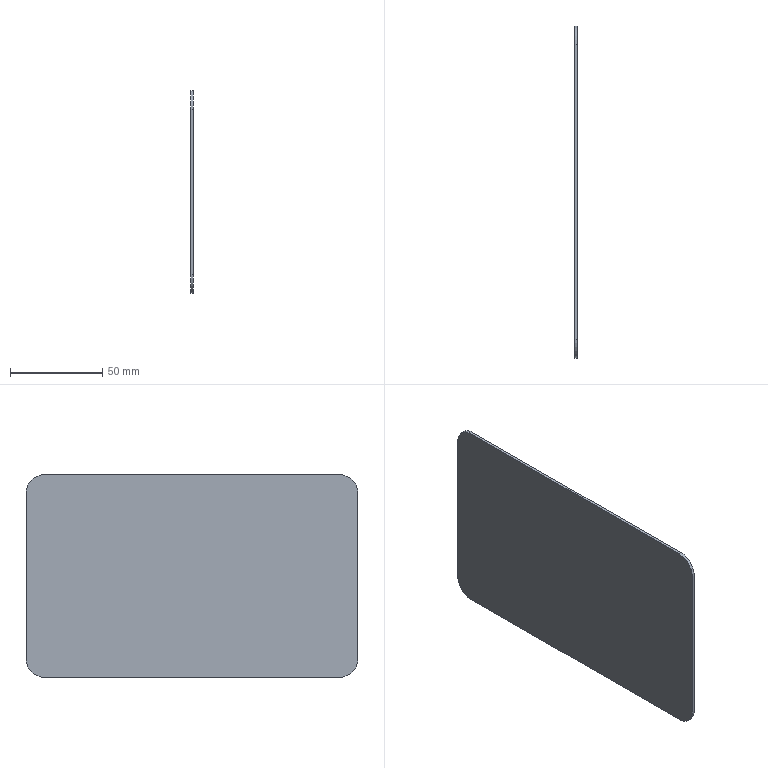Part | STEP file | RJWD-DY-B1_X2_5FEB5E7267DC680_1 | 1 solid | 10 faces | box 1.5 x 180 x 110 mm | volume 29571 mm3 | plane 6 | cylinder 4 | commonest cylinder face diameters 20 x4
STEP:
#1=CARTESIAN_POINT('',(0.,0.,0.));
#2=DIRECTION('',(0.,0.,1.));
#3=DIRECTION('',(1.,0.,0.));
#4=AXIS2_PLACEMENT_3D('',#1,#2,#3);
#5=CARTESIAN_POINT('',(768.8,3170.8,1288.594));
#6=VERTEX_POINT('',#5);
#7=CARTESIAN_POINT('',(768.8,3170.8,1378.594));
#8=VERTEX_POINT('',#7);
#9=CARTESIAN_POINT('',(768.8,3170.8,1288.594));
#10=DIRECTION('',(0.,0.,1.));
#11=VECTOR('',#10,1.);
#12=LINE('',#9,#11);
#13=CARTESIAN_POINT('',(770.3,3170.8,1378.594));
#14=DIRECTION('',(0.,1.,0.));
#15=DIRECTION('',(0.,0.,1.));
#16=AXIS2_PLACEMENT_3D('',#13,#14,#15);
#17=PLANE('',#16);
#18=CARTESIAN_POINT('',(-90.,-1.5));
#19=DIRECTION('',(1.,0.));
#20=VECTOR('',#19,1.);
#21=LINE('',#18,#20);
#22=(GEOMETRIC_REPRESENTATION_CONTEXT(2)PARAMETRIC_REPRESENTATION_CONTEXT()REPRESENTATION_CONTEXT('',''));
#23=DEFINITIONAL_REPRESENTATION('',(#21),#22);
#24=PCURVE('',#17,#23);
#25=CARTESIAN_POINT('',(768.8,3180.8,1288.594));
#26=DIRECTION('',(1.,0.,0.));
#27=DIRECTION('',(0.,0.,-1.));
#28=AXIS2_PLACEMENT_3D('',#25,#26,#27);
#29=PLANE('',#28);
#30=CARTESIAN_POINT('',(0.,-10.));
#31=DIRECTION('',(-1.,0.));
#32=VECTOR('',#31,1.);
#33=LINE('',#30,#32);
#34=(GEOMETRIC_REPRESENTATION_CONTEXT(2)PARAMETRIC_REPRESENTATION_CONTEXT()REPRESENTATION_CONTEXT('',''));
#35=DEFINITIONAL_REPRESENTATION('',(#33),#34);
#36=PCURVE('',#29,#35);
#37=SURFACE_CURVE('',#12,(#24,#36),.PCURVE_S1.);
#38=EDGE_CURVE('',#6,#8,#37,.T.);
#39=ORIENTED_EDGE('',*,*,#38,.T.);
#40=CARTESIAN_POINT('',(770.3,3170.8,1378.594));
#41=VERTEX_POINT('',#40);
#42=CARTESIAN_POINT('',(768.8,3170.8,1378.594));
#43=DIRECTION('',(1.,0.,0.));
#44=VECTOR('',#43,1.);
#45=LINE('',#42,#44);
#46=CARTESIAN_POINT('',(0.,-1.5));
#47=DIRECTION('',(0.,1.));
#48=VECTOR('',#47,1.);
#49=LINE('',#46,#48);
#50=(GEOMETRIC_REPRESENTATION_CONTEXT(2)PARAMETRIC_REPRESENTATION_CONTEXT()REPRESENTATION_CONTEXT('',''));
#51=DEFINITIONAL_REPRESENTATION('',(#49),#50);
#52=PCURVE('',#17,#51);
#53=CARTESIAN_POINT('',(770.3,3180.8,1378.594));
#54=DIRECTION('',(-1.,0.,0.));
#55=DIRECTION('',(0.,0.,1.));
#56=AXIS2_PLACEMENT_3D('',#53,#54,#55);
#57=CYLINDRICAL_SURFACE('',#56,10.);
#58=CARTESIAN_POINT('',(4.712,1.5));
#59=DIRECTION('',(0.,-1.));
#60=VECTOR('',#59,1.);
#61=LINE('',#58,#60);
#62=(GEOMETRIC_REPRESENTATION_CONTEXT(2)PARAMETRIC_REPRESENTATION_CONTEXT()REPRESENTATION_CONTEXT('',''));
#63=DEFINITIONAL_REPRESENTATION('',(#61),#62);
#64=PCURVE('',#57,#63);
#65=SURFACE_CURVE('',#45,(#52,#64),.PCURVE_S1.);
#66=EDGE_CURVE('',#8,#41,#65,.T.);
#67=ORIENTED_EDGE('',*,*,#66,.T.);
#68=CARTESIAN_POINT('',(770.3,3170.8,1288.594));
#69=VERTEX_POINT('',#68);
#70=CARTESIAN_POINT('',(770.3,3170.8,1288.594));
#71=DIRECTION('',(0.,0.,1.));
#72=VECTOR('',#71,1.);
#73=LINE('',#70,#72);
#74=CARTESIAN_POINT('',(-90.,0.));
#75=DIRECTION('',(1.,0.));
#76=VECTOR('',#75,1.);
#77=LINE('',#74,#76);
#78=(GEOMETRIC_REPRESENTATION_CONTEXT(2)PARAMETRIC_REPRESENTATION_CONTEXT()REPRESENTATION_CONTEXT('',''));
#79=DEFINITIONAL_REPRESENTATION('',(#77),#78);
#80=PCURVE('',#17,#79);
#81=CARTESIAN_POINT('',(770.3,3180.8,1288.594));
#82=DIRECTION('',(1.,0.,0.));
#83=DIRECTION('',(0.,0.,-1.));
#84=AXIS2_PLACEMENT_3D('',#81,#82,#83);
#85=PLANE('',#84);
#86=CARTESIAN_POINT('',(0.,-10.));
#87=DIRECTION('',(-1.,0.));
#88=VECTOR('',#87,1.);
#89=LINE('',#86,#88);
#90=(GEOMETRIC_REPRESENTATION_CONTEXT(2)PARAMETRIC_REPRESENTATION_CONTEXT()REPRESENTATION_CONTEXT('',''));
#91=DEFINITIONAL_REPRESENTATION('',(#89),#90);
#92=PCURVE('',#85,#91);
#93=SURFACE_CURVE('',#73,(#80,#92),.PCURVE_S1.);
#94=EDGE_CURVE('',#69,#41,#93,.T.);
#95=ORIENTED_EDGE('',*,*,#94,.F.);
#96=CARTESIAN_POINT('',(770.3,3170.8,1288.594));
#97=DIRECTION('',(-1.,0.,0.));
#98=VECTOR('',#97,1.);
#99=LINE('',#96,#98);
#100=CARTESIAN_POINT('',(-90.,0.));
#101=DIRECTION('',(0.,-1.));
#102=VECTOR('',#101,1.);
#103=LINE('',#100,#102);
#104=(GEOMETRIC_REPRESENTATION_CONTEXT(2)PARAMETRIC_REPRESENTATION_CONTEXT()REPRESENTATION_CONTEXT('',''));
#105=DEFINITIONAL_REPRESENTATION('',(#103),#104);
#106=PCURVE('',#17,#105);
#107=CARTESIAN_POINT('',(770.3,3180.8,1288.594));
#108=DIRECTION('',(-1.,0.,0.));
#109=DIRECTION('',(0.,0.,1.));
#110=AXIS2_PLACEMENT_3D('',#107,#108,#109);
#111=CYLINDRICAL_SURFACE('',#110,10.);
#112=CARTESIAN_POINT('',(4.712,0.));
#113=DIRECTION('',(0.,1.));
#114=VECTOR('',#113,1.);
#115=LINE('',#112,#114);
#116=(GEOMETRIC_REPRESENTATION_CONTEXT(2)PARAMETRIC_REPRESENTATION_CONTEXT()REPRESENTATION_CONTEXT('',''));
#117=DEFINITIONAL_REPRESENTATION('',(#115),#116);
#118=PCURVE('',#111,#117);
#119=SURFACE_CURVE('',#99,(#106,#118),.PCURVE_S1.);
#120=EDGE_CURVE('',#69,#6,#119,.T.);
#121=ORIENTED_EDGE('',*,*,#120,.T.);
#122=EDGE_LOOP('',(#39,#67,#95,#121));
#123=FACE_BOUND('',#122,.F.);
#124=ADVANCED_FACE('',(#123),#17,.F.);
#125=ORIENTED_EDGE('',*,*,#38,.F.);
#126=CARTESIAN_POINT('',(768.8,3180.8,1278.594));
#127=VERTEX_POINT('',#126);
#128=CARTESIAN_POINT('',(768.8,3180.8,1288.594));
#129=DIRECTION('',(-1.,0.,0.));
#130=DIRECTION('',(0.,0.,-1.));
#131=AXIS2_PLACEMENT_3D('',#128,#129,#130);
#132=CIRCLE('',#131,10.);
#133=CARTESIAN_POINT('',(10.,0.));
#134=CARTESIAN_POINT('',(10.,-17.321));
#135=CARTESIAN_POINT('',(-5.,-8.66));
#136=CARTESIAN_POINT('',(-20.,0.));
#137=CARTESIAN_POINT('',(-5.,8.66));
#138=CARTESIAN_POINT('',(10.,17.321));
#139=CARTESIAN_POINT('',(10.,0.));
#140=(BOUNDED_CURVE()B_SPLINE_CURVE(2,(#133,#134,#135,#136,#137,#138,#139),.UNSPECIFIED.,.T.,.F.)B_SPLINE_CURVE_WITH_KNOTS((1,2,2,2,2,1),(-2.094,0.,2.094,4.189,6.283,8.378),.UNSPECIFIED.)CURVE()GEOMETRIC_REPRESENTATION_ITEM()RATIONAL_B_SPLINE_CURVE((1.,0.5,1.,0.5,1.,0.5,1.))REPRESENTATION_ITEM(''));
#141=(GEOMETRIC_REPRESENTATION_CONTEXT(2)PARAMETRIC_REPRESENTATION_CONTEXT()REPRESENTATION_CONTEXT('',''));
#142=DEFINITIONAL_REPRESENTATION('',(#140),#141);
#143=PCURVE('',#29,#142);
#144=CARTESIAN_POINT('',(3.142,1.5));
#145=DIRECTION('',(1.,0.));
#146=VECTOR('',#145,1.);
#147=LINE('',#144,#146);
#148=(GEOMETRIC_REPRESENTATION_CONTEXT(2)PARAMETRIC_REPRESENTATION_CONTEXT()REPRESENTATION_CONTEXT('',''));
#149=DEFINITIONAL_REPRESENTATION('',(#147),#148);
#150=PCURVE('',#111,#149);
#151=SURFACE_CURVE('',#132,(#143,#150),.PCURVE_S1.);
#152=EDGE_CURVE('',#127,#6,#151,.T.);
#153=ORIENTED_EDGE('',*,*,#152,.F.);
#154=CARTESIAN_POINT('',(768.8,3340.8,1278.594));
#155=VERTEX_POINT('',#154);
#156=CARTESIAN_POINT('',(768.8,3340.8,1278.594));
#157=DIRECTION('',(0.,-1.,0.));
#158=VECTOR('',#157,1.);
#159=LINE('',#156,#158);
#160=CARTESIAN_POINT('',(10.,160.));
#161=DIRECTION('',(0.,-1.));
#162=VECTOR('',#161,1.);
#163=LINE('',#160,#162);
#164=(GEOMETRIC_REPRESENTATION_CONTEXT(2)PARAMETRIC_REPRESENTATION_CONTEXT()REPRESENTATION_CONTEXT('',''));
#165=DEFINITIONAL_REPRESENTATION('',(#163),#164);
#166=PCURVE('',#29,#165);
#167=CARTESIAN_POINT('',(770.3,3180.8,1278.594));
#168=DIRECTION('',(0.,0.,1.));
#169=DIRECTION('',(1.,0.,0.));
#170=AXIS2_PLACEMENT_3D('',#167,#168,#169);
#171=PLANE('',#170);
#172=CARTESIAN_POINT('',(-1.5,160.));
#173=DIRECTION('',(0.,-1.));
#174=VECTOR('',#173,1.);
#175=LINE('',#172,#174);
#176=(GEOMETRIC_REPRESENTATION_CONTEXT(2)PARAMETRIC_REPRESENTATION_CONTEXT()REPRESENTATION_CONTEXT('',''));
#177=DEFINITIONAL_REPRESENTATION('',(#175),#176);
#178=PCURVE('',#171,#177);
#179=SURFACE_CURVE('',#159,(#166,#178),.PCURVE_S1.);
#180=EDGE_CURVE('',#155,#127,#179,.T.);
#181=ORIENTED_EDGE('',*,*,#180,.F.);
#182=CARTESIAN_POINT('',(768.8,3350.8,1288.594));
#183=VERTEX_POINT('',#182);
#184=CARTESIAN_POINT('',(768.8,3340.8,1288.594));
#185=DIRECTION('',(-1.,0.,0.));
#186=DIRECTION('',(0.,1.,0.));
#187=AXIS2_PLACEMENT_3D('',#184,#185,#186);
#188=CIRCLE('',#187,10.);
#189=CARTESIAN_POINT('',(0.,170.));
#190=CARTESIAN_POINT('',(17.321,170.));
#191=CARTESIAN_POINT('',(8.66,155.));
#192=CARTESIAN_POINT('',(0.,140.));
#193=CARTESIAN_POINT('',(-8.66,155.));
#194=CARTESIAN_POINT('',(-17.321,170.));
#195=CARTESIAN_POINT('',(0.,170.));
#196=(BOUNDED_CURVE()B_SPLINE_CURVE(2,(#189,#190,#191,#192,#193,#194,#195),.UNSPECIFIED.,.T.,.F.)B_SPLINE_CURVE_WITH_KNOTS((1,2,2,2,2,1),(-2.094,0.,2.094,4.189,6.283,8.378),.UNSPECIFIED.)CURVE()GEOMETRIC_REPRESENTATION_ITEM()RATIONAL_B_SPLINE_CURVE((1.,0.5,1.,0.5,1.,0.5,1.))REPRESENTATION_ITEM(''));
#197=(GEOMETRIC_REPRESENTATION_CONTEXT(2)PARAMETRIC_REPRESENTATION_CONTEXT()REPRESENTATION_CONTEXT('',''));
#198=DEFINITIONAL_REPRESENTATION('',(#196),#197);
#199=PCURVE('',#29,#198);
#200=CARTESIAN_POINT('',(770.3,3340.8,1288.594));
#201=DIRECTION('',(-1.,0.,0.));
#202=DIRECTION('',(0.,0.,1.));
#203=AXIS2_PLACEMENT_3D('',#200,#201,#202);
#204=CYLINDRICAL_SURFACE('',#203,10.);
#205=CARTESIAN_POINT('',(1.571,1.5));
#206=DIRECTION('',(1.,0.));
#207=VECTOR('',#206,1.);
#208=LINE('',#205,#207);
#209=(GEOMETRIC_REPRESENTATION_CONTEXT(2)PARAMETRIC_REPRESENTATION_CONTEXT()REPRESENTATION_CONTEXT('',''));
#210=DEFINITIONAL_REPRESENTATION('',(#208),#209);
#211=PCURVE('',#204,#210);
#212=SURFACE_CURVE('',#188,(#199,#211),.PCURVE_S1.);
#213=EDGE_CURVE('',#183,#155,#212,.T.);
#214=ORIENTED_EDGE('',*,*,#213,.F.);
#215=CARTESIAN_POINT('',(768.8,3350.8,1378.594));
#216=VERTEX_POINT('',#215);
#217=CARTESIAN_POINT('',(768.8,3350.8,1378.594));
#218=DIRECTION('',(0.,0.,-1.));
#219=VECTOR('',#218,1.);
#220=LINE('',#217,#219);
#221=CARTESIAN_POINT('',(-90.,170.));
#222=DIRECTION('',(1.,0.));
#223=VECTOR('',#222,1.);
#224=LINE('',#221,#223);
#225=(GEOMETRIC_REPRESENTATION_CONTEXT(2)PARAMETRIC_REPRESENTATION_CONTEXT()REPRESENTATION_CONTEXT('',''));
#226=DEFINITIONAL_REPRESENTATION('',(#224),#225);
#227=PCURVE('',#29,#226);
#228=CARTESIAN_POINT('',(770.3,3350.8,1288.594));
#229=DIRECTION('',(0.,-1.,0.));
#230=DIRECTION('',(0.,0.,-1.));
#231=AXIS2_PLACEMENT_3D('',#228,#229,#230);
#232=PLANE('',#231);
#233=CARTESIAN_POINT('',(-90.,-1.5));
#234=DIRECTION('',(1.,0.));
#235=VECTOR('',#234,1.);
#236=LINE('',#233,#235);
#237=(GEOMETRIC_REPRESENTATION_CONTEXT(2)PARAMETRIC_REPRESENTATION_CONTEXT()REPRESENTATION_CONTEXT('',''));
#238=DEFINITIONAL_REPRESENTATION('',(#236),#237);
#239=PCURVE('',#232,#238);
#240=SURFACE_CURVE('',#220,(#227,#239),.PCURVE_S1.);
#241=EDGE_CURVE('',#216,#183,#240,.T.);
#242=ORIENTED_EDGE('',*,*,#241,.F.);
#243=CARTESIAN_POINT('',(768.8,3340.8,1388.594));
#244=VERTEX_POINT('',#243);
#245=CARTESIAN_POINT('',(768.8,3340.8,1378.594));
#246=DIRECTION('',(-1.,0.,0.));
#247=DIRECTION('',(0.,0.,1.));
#248=AXIS2_PLACEMENT_3D('',#245,#246,#247);
#249=CIRCLE('',#248,10.);
#250=CARTESIAN_POINT('',(-100.,160.));
#251=CARTESIAN_POINT('',(-100.,177.321));
#252=CARTESIAN_POINT('',(-85.,168.66));
#253=CARTESIAN_POINT('',(-70.,160.));
#254=CARTESIAN_POINT('',(-85.,151.34));
#255=CARTESIAN_POINT('',(-100.,142.679));
#256=CARTESIAN_POINT('',(-100.,160.));
#257=(BOUNDED_CURVE()B_SPLINE_CURVE(2,(#250,#251,#252,#253,#254,#255,#256),.UNSPECIFIED.,.T.,.F.)B_SPLINE_CURVE_WITH_KNOTS((1,2,2,2,2,1),(-2.094,0.,2.094,4.189,6.283,8.378),.UNSPECIFIED.)CURVE()GEOMETRIC_REPRESENTATION_ITEM()RATIONAL_B_SPLINE_CURVE((1.,0.5,1.,0.5,1.,0.5,1.))REPRESENTATION_ITEM(''));
#258=(GEOMETRIC_REPRESENTATION_CONTEXT(2)PARAMETRIC_REPRESENTATION_CONTEXT()REPRESENTATION_CONTEXT('',''));
#259=DEFINITIONAL_REPRESENTATION('',(#257),#258);
#260=PCURVE('',#29,#259);
#261=CARTESIAN_POINT('',(770.3,3340.8,1378.594));
#262=DIRECTION('',(-1.,0.,0.));
#263=DIRECTION('',(0.,0.,1.));
#264=AXIS2_PLACEMENT_3D('',#261,#262,#263);
#265=CYLINDRICAL_SURFACE('',#264,10.);
#266=CARTESIAN_POINT('',(0.,1.5));
#267=DIRECTION('',(1.,0.));
#268=VECTOR('',#267,1.);
#269=LINE('',#266,#268);
#270=(GEOMETRIC_REPRESENTATION_CONTEXT(2)PARAMETRIC_REPRESENTATION_CONTEXT()REPRESENTATION_CONTEXT('',''));
#271=DEFINITIONAL_REPRESENTATION('',(#269),#270);
#272=PCURVE('',#265,#271);
#273=SURFACE_CURVE('',#249,(#260,#272),.PCURVE_S1.);
#274=EDGE_CURVE('',#244,#216,#273,.T.);
#275=ORIENTED_EDGE('',*,*,#274,.F.);
#276=CARTESIAN_POINT('',(768.8,3180.8,1388.594));
#277=VERTEX_POINT('',#276);
#278=CARTESIAN_POINT('',(768.8,3180.8,1388.594));
#279=DIRECTION('',(0.,1.,0.));
#280=VECTOR('',#279,1.);
#281=LINE('',#278,#280);
#282=CARTESIAN_POINT('',(-100.,0.));
#283=DIRECTION('',(0.,1.));
#284=VECTOR('',#283,1.);
#285=LINE('',#282,#284);
#286=(GEOMETRIC_REPRESENTATION_CONTEXT(2)PARAMETRIC_REPRESENTATION_CONTEXT()REPRESENTATION_CONTEXT('',''));
#287=DEFINITIONAL_REPRESENTATION('',(#285),#286);
#288=PCURVE('',#29,#287);
#289=CARTESIAN_POINT('',(770.3,3340.8,1388.594));
#290=DIRECTION('',(0.,0.,-1.));
#291=DIRECTION('',(-1.,0.,0.));
#292=AXIS2_PLACEMENT_3D('',#289,#290,#291);
#293=PLANE('',#292);
#294=CARTESIAN_POINT('',(1.5,-160.));
#295=DIRECTION('',(0.,1.));
#296=VECTOR('',#295,1.);
#297=LINE('',#294,#296);
#298=(GEOMETRIC_REPRESENTATION_CONTEXT(2)PARAMETRIC_REPRESENTATION_CONTEXT()REPRESENTATION_CONTEXT('',''));
#299=DEFINITIONAL_REPRESENTATION('',(#297),#298);
#300=PCURVE('',#293,#299);
#301=SURFACE_CURVE('',#281,(#288,#300),.PCURVE_S1.);
#302=EDGE_CURVE('',#277,#244,#301,.T.);
#303=ORIENTED_EDGE('',*,*,#302,.F.);
#304=CARTESIAN_POINT('',(768.8,3180.8,1378.594));
#305=DIRECTION('',(-1.,0.,0.));
#306=DIRECTION('',(0.,-1.,0.));
#307=AXIS2_PLACEMENT_3D('',#304,#305,#306);
#308=CIRCLE('',#307,10.);
#309=CARTESIAN_POINT('',(-90.,-10.));
#310=CARTESIAN_POINT('',(-107.321,-10.));
#311=CARTESIAN_POINT('',(-98.66,5.));
#312=CARTESIAN_POINT('',(-90.,20.));
#313=CARTESIAN_POINT('',(-81.34,5.));
#314=CARTESIAN_POINT('',(-72.679,-10.));
#315=CARTESIAN_POINT('',(-90.,-10.));
#316=(BOUNDED_CURVE()B_SPLINE_CURVE(2,(#309,#310,#311,#312,#313,#314,#315),.UNSPECIFIED.,.T.,.F.)B_SPLINE_CURVE_WITH_KNOTS((1,2,2,2,2,1),(-2.094,0.,2.094,4.189,6.283,8.378),.UNSPECIFIED.)CURVE()GEOMETRIC_REPRESENTATION_ITEM()RATIONAL_B_SPLINE_CURVE((1.,0.5,1.,0.5,1.,0.5,1.))REPRESENTATION_ITEM(''));
#317=(GEOMETRIC_REPRESENTATION_CONTEXT(2)PARAMETRIC_REPRESENTATION_CONTEXT()REPRESENTATION_CONTEXT('',''));
#318=DEFINITIONAL_REPRESENTATION('',(#316),#317);
#319=PCURVE('',#29,#318);
#320=CARTESIAN_POINT('',(4.712,1.5));
#321=DIRECTION('',(1.,0.));
#322=VECTOR('',#321,1.);
#323=LINE('',#320,#322);
#324=(GEOMETRIC_REPRESENTATION_CONTEXT(2)PARAMETRIC_REPRESENTATION_CONTEXT()REPRESENTATION_CONTEXT('',''));
#325=DEFINITIONAL_REPRESENTATION('',(#323),#324);
#326=PCURVE('',#57,#325);
#327=SURFACE_CURVE('',#308,(#319,#326),.PCURVE_S1.);
#328=EDGE_CURVE('',#8,#277,#327,.T.);
#329=ORIENTED_EDGE('',*,*,#328,.F.);
#330=EDGE_LOOP('',(#125,#153,#181,#214,#242,#275,#303,#329));
#331=FACE_BOUND('',#330,.F.);
#332=ADVANCED_FACE('',(#331),#29,.F.);
#333=CARTESIAN_POINT('',(770.3,3180.8,1278.594));
#334=VERTEX_POINT('',#333);
#335=CARTESIAN_POINT('',(768.8,3180.8,1278.594));
#336=DIRECTION('',(1.,0.,0.));
#337=VECTOR('',#336,1.);
#338=LINE('',#335,#337);
#339=CARTESIAN_POINT('',(3.142,1.5));
#340=DIRECTION('',(0.,-1.));
#341=VECTOR('',#340,1.);
#342=LINE('',#339,#341);
#343=(GEOMETRIC_REPRESENTATION_CONTEXT(2)PARAMETRIC_REPRESENTATION_CONTEXT()REPRESENTATION_CONTEXT('',''));
#344=DEFINITIONAL_REPRESENTATION('',(#342),#343);
#345=PCURVE('',#111,#344);
#346=CARTESIAN_POINT('',(-1.5,0.));
#347=DIRECTION('',(1.,0.));
#348=VECTOR('',#347,1.);
#349=LINE('',#346,#348);
#350=(GEOMETRIC_REPRESENTATION_CONTEXT(2)PARAMETRIC_REPRESENTATION_CONTEXT()REPRESENTATION_CONTEXT('',''));
#351=DEFINITIONAL_REPRESENTATION('',(#349),#350);
#352=PCURVE('',#171,#351);
#353=SURFACE_CURVE('',#338,(#345,#352),.PCURVE_S1.);
#354=EDGE_CURVE('',#127,#334,#353,.T.);
#355=ORIENTED_EDGE('',*,*,#354,.T.);
#356=CARTESIAN_POINT('',(770.3,3180.8,1288.594));
#357=DIRECTION('',(1.,0.,0.));
#358=DIRECTION('',(0.,-1.,0.));
#359=AXIS2_PLACEMENT_3D('',#356,#357,#358);
#360=CIRCLE('',#359,10.);
#361=CARTESIAN_POINT('',(4.712,0.));
#362=DIRECTION('',(-1.,0.));
#363=VECTOR('',#362,1.);
#364=LINE('',#361,#363);
#365=(GEOMETRIC_REPRESENTATION_CONTEXT(2)PARAMETRIC_REPRESENTATION_CONTEXT()REPRESENTATION_CONTEXT('',''));
#366=DEFINITIONAL_REPRESENTATION('',(#364),#365);
#367=PCURVE('',#111,#366);
#368=CARTESIAN_POINT('',(0.,0.));
#369=DIRECTION('',(0.,-1.));
#370=AXIS2_PLACEMENT_2D('',#368,#369);
#371=CIRCLE('',#370,10.);
#372=(GEOMETRIC_REPRESENTATION_CONTEXT(2)PARAMETRIC_REPRESENTATION_CONTEXT()REPRESENTATION_CONTEXT('',''));
#373=DEFINITIONAL_REPRESENTATION('',(#371),#372);
#374=PCURVE('',#85,#373);
#375=SURFACE_CURVE('',#360,(#367,#374),.PCURVE_S1.);
#376=EDGE_CURVE('',#69,#334,#375,.T.);
#377=ORIENTED_EDGE('',*,*,#376,.F.);
#378=ORIENTED_EDGE('',*,*,#120,.T.);
#379=ORIENTED_EDGE('',*,*,#152,.F.);
#380=EDGE_LOOP('',(#355,#377,#378,#379));
#381=FACE_BOUND('',#380,.T.);
#382=ADVANCED_FACE('',(#381),#111,.T.);
#383=ORIENTED_EDGE('',*,*,#94,.T.);
#384=CARTESIAN_POINT('',(770.3,3180.8,1388.594));
#385=VERTEX_POINT('',#384);
#386=CARTESIAN_POINT('',(770.3,3180.8,1378.594));
#387=DIRECTION('',(1.,0.,0.));
#388=DIRECTION('',(0.,0.,1.));
#389=AXIS2_PLACEMENT_3D('',#386,#387,#388);
#390=CIRCLE('',#389,10.);
#391=CARTESIAN_POINT('',(-90.,0.));
#392=DIRECTION('',(-1.,0.));
#393=AXIS2_PLACEMENT_2D('',#391,#392);
#394=CIRCLE('',#393,10.);
#395=(GEOMETRIC_REPRESENTATION_CONTEXT(2)PARAMETRIC_REPRESENTATION_CONTEXT()REPRESENTATION_CONTEXT('',''));
#396=DEFINITIONAL_REPRESENTATION('',(#394),#395);
#397=PCURVE('',#85,#396);
#398=CARTESIAN_POINT('',(6.283,0.));
#399=DIRECTION('',(-1.,0.));
#400=VECTOR('',#399,1.);
#401=LINE('',#398,#400);
#402=(GEOMETRIC_REPRESENTATION_CONTEXT(2)PARAMETRIC_REPRESENTATION_CONTEXT()REPRESENTATION_CONTEXT('',''));
#403=DEFINITIONAL_REPRESENTATION('',(#401),#402);
#404=PCURVE('',#57,#403);
#405=SURFACE_CURVE('',#390,(#397,#404),.PCURVE_S1.);
#406=EDGE_CURVE('',#385,#41,#405,.T.);
#407=ORIENTED_EDGE('',*,*,#406,.F.);
#408=CARTESIAN_POINT('',(770.3,3340.8,1388.594));
#409=VERTEX_POINT('',#408);
#410=CARTESIAN_POINT('',(770.3,3180.8,1388.594));
#411=DIRECTION('',(0.,1.,0.));
#412=VECTOR('',#411,1.);
#413=LINE('',#410,#412);
#414=CARTESIAN_POINT('',(-100.,0.));
#415=DIRECTION('',(0.,1.));
#416=VECTOR('',#415,1.);
#417=LINE('',#414,#416);
#418=(GEOMETRIC_REPRESENTATION_CONTEXT(2)PARAMETRIC_REPRESENTATION_CONTEXT()REPRESENTATION_CONTEXT('',''));
#419=DEFINITIONAL_REPRESENTATION('',(#417),#418);
#420=PCURVE('',#85,#419);
#421=CARTESIAN_POINT('',(0.,-160.));
#422=DIRECTION('',(0.,1.));
#423=VECTOR('',#422,1.);
#424=LINE('',#421,#423);
#425=(GEOMETRIC_REPRESENTATION_CONTEXT(2)PARAMETRIC_REPRESENTATION_CONTEXT()REPRESENTATION_CONTEXT('',''));
#426=DEFINITIONAL_REPRESENTATION('',(#424),#425);
#427=PCURVE('',#293,#426);
#428=SURFACE_CURVE('',#413,(#420,#427),.PCURVE_S1.);
#429=EDGE_CURVE('',#385,#409,#428,.T.);
#430=ORIENTED_EDGE('',*,*,#429,.T.);
#431=CARTESIAN_POINT('',(770.3,3350.8,1378.594));
#432=VERTEX_POINT('',#431);
#433=CARTESIAN_POINT('',(770.3,3340.8,1378.594));
#434=DIRECTION('',(1.,0.,0.));
#435=DIRECTION('',(0.,1.,0.));
#436=AXIS2_PLACEMENT_3D('',#433,#434,#435);
#437=CIRCLE('',#436,10.);
#438=CARTESIAN_POINT('',(-90.,160.));
#439=DIRECTION('',(0.,1.));
#440=AXIS2_PLACEMENT_2D('',#438,#439);
#441=CIRCLE('',#440,10.);
#442=(GEOMETRIC_REPRESENTATION_CONTEXT(2)PARAMETRIC_REPRESENTATION_CONTEXT()REPRESENTATION_CONTEXT('',''));
#443=DEFINITIONAL_REPRESENTATION('',(#441),#442);
#444=PCURVE('',#85,#443);
#445=CARTESIAN_POINT('',(1.571,0.));
#446=DIRECTION('',(-1.,0.));
#447=VECTOR('',#446,1.);
#448=LINE('',#445,#447);
#449=(GEOMETRIC_REPRESENTATION_CONTEXT(2)PARAMETRIC_REPRESENTATION_CONTEXT()REPRESENTATION_CONTEXT('',''));
#450=DEFINITIONAL_REPRESENTATION('',(#448),#449);
#451=PCURVE('',#265,#450);
#452=SURFACE_CURVE('',#437,(#444,#451),.PCURVE_S1.);
#453=EDGE_CURVE('',#432,#409,#452,.T.);
#454=ORIENTED_EDGE('',*,*,#453,.F.);
#455=CARTESIAN_POINT('',(770.3,3350.8,1288.594));
#456=VERTEX_POINT('',#455);
#457=CARTESIAN_POINT('',(770.3,3350.8,1378.594));
#458=DIRECTION('',(0.,0.,-1.));
#459=VECTOR('',#458,1.);
#460=LINE('',#457,#459);
#461=CARTESIAN_POINT('',(-90.,170.));
#462=DIRECTION('',(1.,0.));
#463=VECTOR('',#462,1.);
#464=LINE('',#461,#463);
#465=(GEOMETRIC_REPRESENTATION_CONTEXT(2)PARAMETRIC_REPRESENTATION_CONTEXT()REPRESENTATION_CONTEXT('',''));
#466=DEFINITIONAL_REPRESENTATION('',(#464),#465);
#467=PCURVE('',#85,#466);
#468=CARTESIAN_POINT('',(-90.,0.));
#469=DIRECTION('',(1.,0.));
#470=VECTOR('',#469,1.);
#471=LINE('',#468,#470);
#472=(GEOMETRIC_REPRESENTATION_CONTEXT(2)PARAMETRIC_REPRESENTATION_CONTEXT()REPRESENTATION_CONTEXT('',''));
#473=DEFINITIONAL_REPRESENTATION('',(#471),#472);
#474=PCURVE('',#232,#473);
#475=SURFACE_CURVE('',#460,(#467,#474),.PCURVE_S1.);
#476=EDGE_CURVE('',#432,#456,#475,.T.);
#477=ORIENTED_EDGE('',*,*,#476,.T.);
#478=CARTESIAN_POINT('',(770.3,3340.8,1278.594));
#479=VERTEX_POINT('',#478);
#480=CARTESIAN_POINT('',(770.3,3340.8,1288.594));
#481=DIRECTION('',(1.,0.,0.));
#482=DIRECTION('',(0.,0.,-1.));
#483=AXIS2_PLACEMENT_3D('',#480,#481,#482);
#484=CIRCLE('',#483,10.);
#485=CARTESIAN_POINT('',(0.,160.));
#486=DIRECTION('',(1.,0.));
#487=AXIS2_PLACEMENT_2D('',#485,#486);
#488=CIRCLE('',#487,10.);
#489=(GEOMETRIC_REPRESENTATION_CONTEXT(2)PARAMETRIC_REPRESENTATION_CONTEXT()REPRESENTATION_CONTEXT('',''));
#490=DEFINITIONAL_REPRESENTATION('',(#488),#489);
#491=PCURVE('',#85,#490);
#492=CARTESIAN_POINT('',(3.142,0.));
#493=DIRECTION('',(-1.,0.));
#494=VECTOR('',#493,1.);
#495=LINE('',#492,#494);
#496=(GEOMETRIC_REPRESENTATION_CONTEXT(2)PARAMETRIC_REPRESENTATION_CONTEXT()REPRESENTATION_CONTEXT('',''));
#497=DEFINITIONAL_REPRESENTATION('',(#495),#496);
#498=PCURVE('',#204,#497);
#499=SURFACE_CURVE('',#484,(#491,#498),.PCURVE_S1.);
#500=EDGE_CURVE('',#479,#456,#499,.T.);
#501=ORIENTED_EDGE('',*,*,#500,.F.);
#502=CARTESIAN_POINT('',(770.3,3340.8,1278.594));
#503=DIRECTION('',(0.,-1.,0.));
#504=VECTOR('',#503,1.);
#505=LINE('',#502,#504);
#506=CARTESIAN_POINT('',(10.,160.));
#507=DIRECTION('',(0.,-1.));
#508=VECTOR('',#507,1.);
#509=LINE('',#506,#508);
#510=(GEOMETRIC_REPRESENTATION_CONTEXT(2)PARAMETRIC_REPRESENTATION_CONTEXT()REPRESENTATION_CONTEXT('',''));
#511=DEFINITIONAL_REPRESENTATION('',(#509),#510);
#512=PCURVE('',#85,#511);
#513=CARTESIAN_POINT('',(0.,160.));
#514=DIRECTION('',(0.,-1.));
#515=VECTOR('',#514,1.);
#516=LINE('',#513,#515);
#517=(GEOMETRIC_REPRESENTATION_CONTEXT(2)PARAMETRIC_REPRESENTATION_CONTEXT()REPRESENTATION_CONTEXT('',''));
#518=DEFINITIONAL_REPRESENTATION('',(#516),#517);
#519=PCURVE('',#171,#518);
#520=SURFACE_CURVE('',#505,(#512,#519),.PCURVE_S1.);
#521=EDGE_CURVE('',#479,#334,#520,.T.);
#522=ORIENTED_EDGE('',*,*,#521,.T.);
#523=ORIENTED_EDGE('',*,*,#376,.F.);
#524=EDGE_LOOP('',(#383,#407,#430,#454,#477,#501,#522,#523));
#525=FACE_BOUND('',#524,.F.);
#526=ADVANCED_FACE('',(#525),#85,.T.);
#527=ORIENTED_EDGE('',*,*,#66,.T.);
#528=ORIENTED_EDGE('',*,*,#406,.F.);
#529=CARTESIAN_POINT('',(770.3,3180.8,1388.594));
#530=DIRECTION('',(-1.,0.,0.));
#531=VECTOR('',#530,1.);
#532=LINE('',#529,#531);
#533=CARTESIAN_POINT('',(6.283,0.));
#534=DIRECTION('',(0.,1.));
#535=VECTOR('',#534,1.);
#536=LINE('',#533,#535);
#537=(GEOMETRIC_REPRESENTATION_CONTEXT(2)PARAMETRIC_REPRESENTATION_CONTEXT()REPRESENTATION_CONTEXT('',''));
#538=DEFINITIONAL_REPRESENTATION('',(#536),#537);
#539=PCURVE('',#57,#538);
#540=CARTESIAN_POINT('',(0.,-160.));
#541=DIRECTION('',(1.,0.));
#542=VECTOR('',#541,1.);
#543=LINE('',#540,#542);
#544=(GEOMETRIC_REPRESENTATION_CONTEXT(2)PARAMETRIC_REPRESENTATION_CONTEXT()REPRESENTATION_CONTEXT('',''));
#545=DEFINITIONAL_REPRESENTATION('',(#543),#544);
#546=PCURVE('',#293,#545);
#547=SURFACE_CURVE('',#532,(#539,#546),.PCURVE_S1.);
#548=EDGE_CURVE('',#385,#277,#547,.T.);
#549=ORIENTED_EDGE('',*,*,#548,.T.);
#550=ORIENTED_EDGE('',*,*,#328,.F.);
#551=EDGE_LOOP('',(#527,#528,#549,#550));
#552=FACE_BOUND('',#551,.T.);
#553=ADVANCED_FACE('',(#552),#57,.T.);
#554=ORIENTED_EDGE('',*,*,#302,.T.);
#555=CARTESIAN_POINT('',(768.8,3340.8,1388.594));
#556=DIRECTION('',(1.,0.,0.));
#557=VECTOR('',#556,1.);
#558=LINE('',#555,#557);
#559=CARTESIAN_POINT('',(1.5,0.));
#560=DIRECTION('',(-1.,0.));
#561=VECTOR('',#560,1.);
#562=LINE('',#559,#561);
#563=(GEOMETRIC_REPRESENTATION_CONTEXT(2)PARAMETRIC_REPRESENTATION_CONTEXT()REPRESENTATION_CONTEXT('',''));
#564=DEFINITIONAL_REPRESENTATION('',(#562),#563);
#565=PCURVE('',#293,#564);
#566=CARTESIAN_POINT('',(0.,1.5));
#567=CARTESIAN_POINT('',(0.,1.477));
#568=CARTESIAN_POINT('',(0.,1.432));
#569=CARTESIAN_POINT('',(0.,1.364));
#570=CARTESIAN_POINT('',(0.,1.295));
#571=CARTESIAN_POINT('',(0.,1.227));
#572=CARTESIAN_POINT('',(0.,1.159));
#573=CARTESIAN_POINT('',(0.,1.091));
#574=CARTESIAN_POINT('',(0.,1.023));
#575=CARTESIAN_POINT('',(0.,0.9545));
#576=CARTESIAN_POINT('',(0.,0.8864));
#577=CARTESIAN_POINT('',(0.,0.8182));
#578=CARTESIAN_POINT('',(0.,0.75));
#579=CARTESIAN_POINT('',(0.,0.6818));
#580=CARTESIAN_POINT('',(0.,0.6136));
#581=CARTESIAN_POINT('',(0.,0.5455));
#582=CARTESIAN_POINT('',(0.,0.4773));
#583=CARTESIAN_POINT('',(0.,0.4091));
#584=CARTESIAN_POINT('',(0.,0.3409));
#585=CARTESIAN_POINT('',(0.,0.2727));
#586=CARTESIAN_POINT('',(0.,0.2045));
#587=CARTESIAN_POINT('',(0.,0.1364));
#588=CARTESIAN_POINT('',(0.,0.06818));
#589=CARTESIAN_POINT('',(0.,0.02273));
#590=CARTESIAN_POINT('',(0.,0.));
#591=B_SPLINE_CURVE_WITH_KNOTS('',3,(#566,#567,#568,#569,#570,#571,#572,#573,#574,#575,#576,#577,#578,#579,#580,#581,#582,#583,#584,#585,#586,#587,#588,#589,#590),.UNSPECIFIED.,.F.,.F.,(4,1,1,1,1,1,1,1,1,1,1,1,1,1,1,1,1,1,1,1,1,1,4),(0.,0.06818,0.1364,0.2045,0.2727,0.3409,0.4091,0.4773,0.5455,0.6136,0.6818,0.75,0.8182,0.8864,0.9545,1.023,1.091,1.159,1.227,1.295,1.364,1.432,1.5),.QUASI_UNIFORM_KNOTS.);
#592=(GEOMETRIC_REPRESENTATION_CONTEXT(2)PARAMETRIC_REPRESENTATION_CONTEXT()REPRESENTATION_CONTEXT('',''));
#593=DEFINITIONAL_REPRESENTATION('',(#591),#592);
#594=PCURVE('',#265,#593);
#595=SURFACE_CURVE('',#558,(#565,#594),.PCURVE_S1.);
#596=EDGE_CURVE('',#244,#409,#595,.T.);
#597=ORIENTED_EDGE('',*,*,#596,.T.);
#598=ORIENTED_EDGE('',*,*,#429,.F.);
#599=ORIENTED_EDGE('',*,*,#548,.T.);
#600=EDGE_LOOP('',(#554,#597,#598,#599));
#601=FACE_BOUND('',#600,.F.);
#602=ADVANCED_FACE('',(#601),#293,.F.);
#603=ORIENTED_EDGE('',*,*,#596,.T.);
#604=ORIENTED_EDGE('',*,*,#453,.F.);
#605=CARTESIAN_POINT('',(770.3,3350.8,1378.594));
#606=DIRECTION('',(-1.,0.,0.));
#607=VECTOR('',#606,1.);
#608=LINE('',#605,#607);
#609=CARTESIAN_POINT('',(1.571,0.));
#610=DIRECTION('',(0.,1.));
#611=VECTOR('',#610,1.);
#612=LINE('',#609,#611);
#613=(GEOMETRIC_REPRESENTATION_CONTEXT(2)PARAMETRIC_REPRESENTATION_CONTEXT()REPRESENTATION_CONTEXT('',''));
#614=DEFINITIONAL_REPRESENTATION('',(#612),#613);
#615=PCURVE('',#265,#614);
#616=CARTESIAN_POINT('',(-90.,0.));
#617=DIRECTION('',(0.,-1.));
#618=VECTOR('',#617,1.);
#619=LINE('',#616,#618);
#620=(GEOMETRIC_REPRESENTATION_CONTEXT(2)PARAMETRIC_REPRESENTATION_CONTEXT()REPRESENTATION_CONTEXT('',''));
#621=DEFINITIONAL_REPRESENTATION('',(#619),#620);
#622=PCURVE('',#232,#621);
#623=SURFACE_CURVE('',#608,(#615,#622),.PCURVE_S1.);
#624=EDGE_CURVE('',#432,#216,#623,.T.);
#625=ORIENTED_EDGE('',*,*,#624,.T.);
#626=ORIENTED_EDGE('',*,*,#274,.F.);
#627=EDGE_LOOP('',(#603,#604,#625,#626));
#628=FACE_BOUND('',#627,.T.);
#629=ADVANCED_FACE('',(#628),#265,.T.);
#630=ORIENTED_EDGE('',*,*,#241,.T.);
#631=CARTESIAN_POINT('',(768.8,3350.8,1288.594));
#632=DIRECTION('',(1.,0.,0.));
#633=VECTOR('',#632,1.);
#634=LINE('',#631,#633);
#635=CARTESIAN_POINT('',(0.,-1.5));
#636=DIRECTION('',(0.,1.));
#637=VECTOR('',#636,1.);
#638=LINE('',#635,#637);
#639=(GEOMETRIC_REPRESENTATION_CONTEXT(2)PARAMETRIC_REPRESENTATION_CONTEXT()REPRESENTATION_CONTEXT('',''));
#640=DEFINITIONAL_REPRESENTATION('',(#638),#639);
#641=PCURVE('',#232,#640);
#642=CARTESIAN_POINT('',(1.571,1.5));
#643=DIRECTION('',(0.,-1.));
#644=VECTOR('',#643,1.);
#645=LINE('',#642,#644);
#646=(GEOMETRIC_REPRESENTATION_CONTEXT(2)PARAMETRIC_REPRESENTATION_CONTEXT()REPRESENTATION_CONTEXT('',''));
#647=DEFINITIONAL_REPRESENTATION('',(#645),#646);
#648=PCURVE('',#204,#647);
#649=SURFACE_CURVE('',#634,(#641,#648),.PCURVE_S1.);
#650=EDGE_CURVE('',#183,#456,#649,.T.);
#651=ORIENTED_EDGE('',*,*,#650,.T.);
#652=ORIENTED_EDGE('',*,*,#476,.F.);
#653=ORIENTED_EDGE('',*,*,#624,.T.);
#654=EDGE_LOOP('',(#630,#651,#652,#653));
#655=FACE_BOUND('',#654,.F.);
#656=ADVANCED_FACE('',(#655),#232,.F.);
#657=ORIENTED_EDGE('',*,*,#650,.T.);
#658=ORIENTED_EDGE('',*,*,#500,.F.);
#659=CARTESIAN_POINT('',(770.3,3340.8,1278.594));
#660=DIRECTION('',(-1.,0.,0.));
#661=VECTOR('',#660,1.);
#662=LINE('',#659,#661);
#663=CARTESIAN_POINT('',(3.142,0.));
#664=DIRECTION('',(0.,1.));
#665=VECTOR('',#664,1.);
#666=LINE('',#663,#665);
#667=(GEOMETRIC_REPRESENTATION_CONTEXT(2)PARAMETRIC_REPRESENTATION_CONTEXT()REPRESENTATION_CONTEXT('',''));
#668=DEFINITIONAL_REPRESENTATION('',(#666),#667);
#669=PCURVE('',#204,#668);
#670=CARTESIAN_POINT('',(0.,160.));
#671=DIRECTION('',(-1.,0.));
#672=VECTOR('',#671,1.);
#673=LINE('',#670,#672);
#674=(GEOMETRIC_REPRESENTATION_CONTEXT(2)PARAMETRIC_REPRESENTATION_CONTEXT()REPRESENTATION_CONTEXT('',''));
#675=DEFINITIONAL_REPRESENTATION('',(#673),#674);
#676=PCURVE('',#171,#675);
#677=SURFACE_CURVE('',#662,(#669,#676),.PCURVE_S1.);
#678=EDGE_CURVE('',#479,#155,#677,.T.);
#679=ORIENTED_EDGE('',*,*,#678,.T.);
#680=ORIENTED_EDGE('',*,*,#213,.F.);
#681=EDGE_LOOP('',(#657,#658,#679,#680));
#682=FACE_BOUND('',#681,.T.);
#683=ADVANCED_FACE('',(#682),#204,.T.);
#684=ORIENTED_EDGE('',*,*,#180,.T.);
#685=ORIENTED_EDGE('',*,*,#354,.T.);
#686=ORIENTED_EDGE('',*,*,#521,.F.);
#687=ORIENTED_EDGE('',*,*,#678,.T.);
#688=EDGE_LOOP('',(#684,#685,#686,#687));
#689=FACE_BOUND('',#688,.F.);
#690=ADVANCED_FACE('',(#689),#171,.F.);
#691=CLOSED_SHELL('',(#124,#332,#382,#526,#553,#602,#629,#656,#683,#690));
#692=MANIFOLD_SOLID_BREP('',#691);
#693=(LENGTH_UNIT()NAMED_UNIT(*)SI_UNIT(.MILLI.,.METRE.));
#694=UNCERTAINTY_MEASURE_WITH_UNIT(LENGTH_MEASURE(0.0000001),#693,'','');
#695=(NAMED_UNIT(*)PLANE_ANGLE_UNIT()SI_UNIT($,.RADIAN.));
#696=(NAMED_UNIT(*)SI_UNIT($,.STERADIAN.)SOLID_ANGLE_UNIT());
#697=(GEOMETRIC_REPRESENTATION_CONTEXT(3)GLOBAL_UNCERTAINTY_ASSIGNED_CONTEXT((#694))GLOBAL_UNIT_ASSIGNED_CONTEXT((#693,#695,#696))REPRESENTATION_CONTEXT('',''));
#698=ADVANCED_BREP_SHAPE_REPRESENTATION('',(#4,#692),#697);